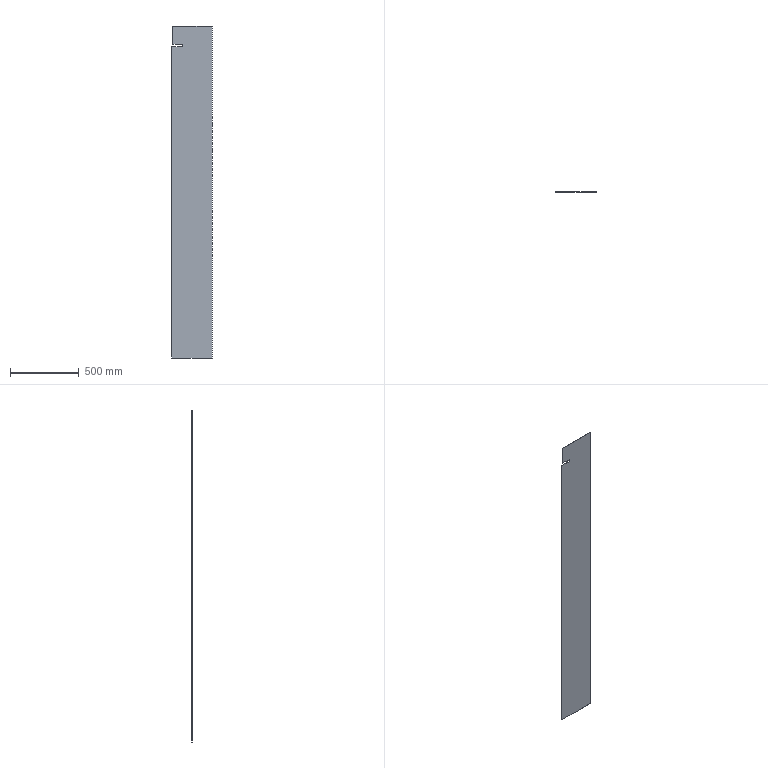Part | STEP file | E3-中转釜花纹Plate 2 | 1 solid | 11 faces | box 296 x 3 x 2420 mm | volume 2142114 mm3 | plane 10 | cylinder 1 | commonest cylinder face diameters 6 x1
STEP:
#1=CARTESIAN_POINT('',(0.,0.,0.));
#2=DIRECTION('',(0.,0.,1.));
#3=DIRECTION('',(1.,0.,0.));
#4=AXIS2_PLACEMENT_3D('',#1,#2,#3);
#5=CARTESIAN_POINT('',(0.,3.,2268.));
#6=VERTEX_POINT('',#5);
#7=CARTESIAN_POINT('',(0.,3.,0.));
#8=VERTEX_POINT('',#7);
#9=CARTESIAN_POINT('',(0.,3.,0.));
#10=DIRECTION('',(0.,0.,-1.));
#11=VECTOR('',#10,1.);
#12=LINE('',#9,#11);
#13=CARTESIAN_POINT('',(0.,3.,0.));
#14=DIRECTION('',(1.,0.,0.));
#15=DIRECTION('',(0.,0.,1.));
#16=AXIS2_PLACEMENT_3D('',#13,#14,#15);
#17=PLANE('',#16);
#18=CARTESIAN_POINT('',(0.,0.));
#19=DIRECTION('',(-1.,0.));
#20=VECTOR('',#19,1.);
#21=LINE('',#18,#20);
#22=(GEOMETRIC_REPRESENTATION_CONTEXT(2)PARAMETRIC_REPRESENTATION_CONTEXT()REPRESENTATION_CONTEXT('',''));
#23=DEFINITIONAL_REPRESENTATION('',(#21),#22);
#24=PCURVE('',#17,#23);
#25=CARTESIAN_POINT('',(0.,3.,0.));
#26=DIRECTION('',(0.,-1.,0.));
#27=DIRECTION('',(0.,0.,1.));
#28=AXIS2_PLACEMENT_3D('',#25,#26,#27);
#29=PLANE('',#28);
#30=CARTESIAN_POINT('',(0.,0.));
#31=DIRECTION('',(-1.,0.));
#32=VECTOR('',#31,1.);
#33=LINE('',#30,#32);
#34=(GEOMETRIC_REPRESENTATION_CONTEXT(2)PARAMETRIC_REPRESENTATION_CONTEXT()REPRESENTATION_CONTEXT('',''));
#35=DEFINITIONAL_REPRESENTATION('',(#33),#34);
#36=PCURVE('',#29,#35);
#37=SURFACE_CURVE('',#12,(#24,#36),.PCURVE_S1.);
#38=EDGE_CURVE('',#6,#8,#37,.T.);
#39=ORIENTED_EDGE('',*,*,#38,.T.);
#40=CARTESIAN_POINT('',(0.,0.,0.));
#41=VERTEX_POINT('',#40);
#42=CARTESIAN_POINT('',(0.,3.,0.));
#43=DIRECTION('',(0.,-1.,0.));
#44=VECTOR('',#43,1.);
#45=LINE('',#42,#44);
#46=CARTESIAN_POINT('',(0.,0.));
#47=DIRECTION('',(0.,1.));
#48=VECTOR('',#47,1.);
#49=LINE('',#46,#48);
#50=(GEOMETRIC_REPRESENTATION_CONTEXT(2)PARAMETRIC_REPRESENTATION_CONTEXT()REPRESENTATION_CONTEXT('',''));
#51=DEFINITIONAL_REPRESENTATION('',(#49),#50);
#52=PCURVE('',#17,#51);
#53=CARTESIAN_POINT('',(0.,3.,0.));
#54=DIRECTION('',(0.,0.,1.));
#55=DIRECTION('',(-1.,0.,0.));
#56=AXIS2_PLACEMENT_3D('',#53,#54,#55);
#57=PLANE('',#56);
#58=CARTESIAN_POINT('',(0.,0.));
#59=DIRECTION('',(0.,1.));
#60=VECTOR('',#59,1.);
#61=LINE('',#58,#60);
#62=(GEOMETRIC_REPRESENTATION_CONTEXT(2)PARAMETRIC_REPRESENTATION_CONTEXT()REPRESENTATION_CONTEXT('',''));
#63=DEFINITIONAL_REPRESENTATION('',(#61),#62);
#64=PCURVE('',#57,#63);
#65=SURFACE_CURVE('',#45,(#52,#64),.PCURVE_S1.);
#66=EDGE_CURVE('',#8,#41,#65,.T.);
#67=ORIENTED_EDGE('',*,*,#66,.T.);
#68=CARTESIAN_POINT('',(0.,0.,2268.));
#69=VERTEX_POINT('',#68);
#70=CARTESIAN_POINT('',(0.,0.,0.));
#71=DIRECTION('',(0.,0.,-1.));
#72=VECTOR('',#71,1.);
#73=LINE('',#70,#72);
#74=CARTESIAN_POINT('',(0.,3.));
#75=DIRECTION('',(-1.,0.));
#76=VECTOR('',#75,1.);
#77=LINE('',#74,#76);
#78=(GEOMETRIC_REPRESENTATION_CONTEXT(2)PARAMETRIC_REPRESENTATION_CONTEXT()REPRESENTATION_CONTEXT('',''));
#79=DEFINITIONAL_REPRESENTATION('',(#77),#78);
#80=PCURVE('',#17,#79);
#81=CARTESIAN_POINT('',(0.,0.,0.));
#82=DIRECTION('',(0.,-1.,0.));
#83=DIRECTION('',(0.,0.,1.));
#84=AXIS2_PLACEMENT_3D('',#81,#82,#83);
#85=PLANE('',#84);
#86=CARTESIAN_POINT('',(0.,0.));
#87=DIRECTION('',(-1.,0.));
#88=VECTOR('',#87,1.);
#89=LINE('',#86,#88);
#90=(GEOMETRIC_REPRESENTATION_CONTEXT(2)PARAMETRIC_REPRESENTATION_CONTEXT()REPRESENTATION_CONTEXT('',''));
#91=DEFINITIONAL_REPRESENTATION('',(#89),#90);
#92=PCURVE('',#85,#91);
#93=SURFACE_CURVE('',#73,(#80,#92),.PCURVE_S1.);
#94=EDGE_CURVE('',#69,#41,#93,.T.);
#95=ORIENTED_EDGE('',*,*,#94,.F.);
#96=CARTESIAN_POINT('',(0.,3.,2268.));
#97=DIRECTION('',(0.,-1.,0.));
#98=VECTOR('',#97,1.);
#99=LINE('',#96,#98);
#100=CARTESIAN_POINT('',(2268.,0.));
#101=DIRECTION('',(0.,1.));
#102=VECTOR('',#101,1.);
#103=LINE('',#100,#102);
#104=(GEOMETRIC_REPRESENTATION_CONTEXT(2)PARAMETRIC_REPRESENTATION_CONTEXT()REPRESENTATION_CONTEXT('',''));
#105=DEFINITIONAL_REPRESENTATION('',(#103),#104);
#106=PCURVE('',#17,#105);
#107=CARTESIAN_POINT('',(-82.,-600.,2268.));
#108=DIRECTION('',(0.,0.,-1.));
#109=DIRECTION('',(1.,0.,0.));
#110=AXIS2_PLACEMENT_3D('',#107,#108,#109);
#111=PLANE('',#110);
#112=CARTESIAN_POINT('',(82.,-603.));
#113=DIRECTION('',(0.,1.));
#114=VECTOR('',#113,1.);
#115=LINE('',#112,#114);
#116=(GEOMETRIC_REPRESENTATION_CONTEXT(2)PARAMETRIC_REPRESENTATION_CONTEXT()REPRESENTATION_CONTEXT('',''));
#117=DEFINITIONAL_REPRESENTATION('',(#115),#116);
#118=PCURVE('',#111,#117);
#119=SURFACE_CURVE('',#99,(#106,#118),.PCURVE_S1.);
#120=EDGE_CURVE('',#6,#69,#119,.T.);
#121=ORIENTED_EDGE('',*,*,#120,.F.);
#122=EDGE_LOOP('',(#39,#67,#95,#121));
#123=FACE_BOUND('',#122,.T.);
#124=ADVANCED_FACE('',(#123),#17,.F.);
#125=CARTESIAN_POINT('',(296.,0.,0.));
#126=VERTEX_POINT('',#125);
#127=CARTESIAN_POINT('',(0.,0.,0.));
#128=DIRECTION('',(1.,0.,0.));
#129=VECTOR('',#128,1.);
#130=LINE('',#127,#129);
#131=CARTESIAN_POINT('',(0.,3.));
#132=DIRECTION('',(-1.,0.));
#133=VECTOR('',#132,1.);
#134=LINE('',#131,#133);
#135=(GEOMETRIC_REPRESENTATION_CONTEXT(2)PARAMETRIC_REPRESENTATION_CONTEXT()REPRESENTATION_CONTEXT('',''));
#136=DEFINITIONAL_REPRESENTATION('',(#134),#135);
#137=PCURVE('',#57,#136);
#138=CARTESIAN_POINT('',(0.,0.));
#139=DIRECTION('',(0.,-1.));
#140=VECTOR('',#139,1.);
#141=LINE('',#138,#140);
#142=(GEOMETRIC_REPRESENTATION_CONTEXT(2)PARAMETRIC_REPRESENTATION_CONTEXT()REPRESENTATION_CONTEXT('',''));
#143=DEFINITIONAL_REPRESENTATION('',(#141),#142);
#144=PCURVE('',#85,#143);
#145=SURFACE_CURVE('',#130,(#137,#144),.PCURVE_S1.);
#146=EDGE_CURVE('',#41,#126,#145,.T.);
#147=ORIENTED_EDGE('',*,*,#146,.F.);
#148=ORIENTED_EDGE('',*,*,#66,.F.);
#149=CARTESIAN_POINT('',(296.,3.,0.));
#150=VERTEX_POINT('',#149);
#151=CARTESIAN_POINT('',(0.,3.,0.));
#152=DIRECTION('',(1.,0.,0.));
#153=VECTOR('',#152,1.);
#154=LINE('',#151,#153);
#155=CARTESIAN_POINT('',(0.,0.));
#156=DIRECTION('',(-1.,0.));
#157=VECTOR('',#156,1.);
#158=LINE('',#155,#157);
#159=(GEOMETRIC_REPRESENTATION_CONTEXT(2)PARAMETRIC_REPRESENTATION_CONTEXT()REPRESENTATION_CONTEXT('',''));
#160=DEFINITIONAL_REPRESENTATION('',(#158),#159);
#161=PCURVE('',#57,#160);
#162=CARTESIAN_POINT('',(0.,0.));
#163=DIRECTION('',(0.,-1.));
#164=VECTOR('',#163,1.);
#165=LINE('',#162,#164);
#166=(GEOMETRIC_REPRESENTATION_CONTEXT(2)PARAMETRIC_REPRESENTATION_CONTEXT()REPRESENTATION_CONTEXT('',''));
#167=DEFINITIONAL_REPRESENTATION('',(#165),#166);
#168=PCURVE('',#29,#167);
#169=SURFACE_CURVE('',#154,(#161,#168),.PCURVE_S1.);
#170=EDGE_CURVE('',#8,#150,#169,.T.);
#171=ORIENTED_EDGE('',*,*,#170,.T.);
#172=CARTESIAN_POINT('',(296.,3.,0.));
#173=DIRECTION('',(0.,-1.,0.));
#174=VECTOR('',#173,1.);
#175=LINE('',#172,#174);
#176=CARTESIAN_POINT('',(-296.,0.));
#177=DIRECTION('',(0.,1.));
#178=VECTOR('',#177,1.);
#179=LINE('',#176,#178);
#180=(GEOMETRIC_REPRESENTATION_CONTEXT(2)PARAMETRIC_REPRESENTATION_CONTEXT()REPRESENTATION_CONTEXT('',''));
#181=DEFINITIONAL_REPRESENTATION('',(#179),#180);
#182=PCURVE('',#57,#181);
#183=CARTESIAN_POINT('',(296.,3.,0.));
#184=DIRECTION('',(-1.,0.,0.));
#185=DIRECTION('',(0.,0.,-1.));
#186=AXIS2_PLACEMENT_3D('',#183,#184,#185);
#187=PLANE('',#186);
#188=CARTESIAN_POINT('',(0.,0.));
#189=DIRECTION('',(0.,1.));
#190=VECTOR('',#189,1.);
#191=LINE('',#188,#190);
#192=(GEOMETRIC_REPRESENTATION_CONTEXT(2)PARAMETRIC_REPRESENTATION_CONTEXT()REPRESENTATION_CONTEXT('',''));
#193=DEFINITIONAL_REPRESENTATION('',(#191),#192);
#194=PCURVE('',#187,#193);
#195=SURFACE_CURVE('',#175,(#182,#194),.PCURVE_S1.);
#196=EDGE_CURVE('',#150,#126,#195,.T.);
#197=ORIENTED_EDGE('',*,*,#196,.T.);
#198=EDGE_LOOP('',(#147,#148,#171,#197));
#199=FACE_BOUND('',#198,.T.);
#200=ADVANCED_FACE('',(#199),#57,.F.);
#201=CARTESIAN_POINT('',(296.,0.,2420.));
#202=VERTEX_POINT('',#201);
#203=CARTESIAN_POINT('',(296.,0.,0.));
#204=DIRECTION('',(0.,0.,1.));
#205=VECTOR('',#204,1.);
#206=LINE('',#203,#205);
#207=CARTESIAN_POINT('',(0.,3.));
#208=DIRECTION('',(-1.,0.));
#209=VECTOR('',#208,1.);
#210=LINE('',#207,#209);
#211=(GEOMETRIC_REPRESENTATION_CONTEXT(2)PARAMETRIC_REPRESENTATION_CONTEXT()REPRESENTATION_CONTEXT('',''));
#212=DEFINITIONAL_REPRESENTATION('',(#210),#211);
#213=PCURVE('',#187,#212);
#214=CARTESIAN_POINT('',(0.,-296.));
#215=DIRECTION('',(1.,0.));
#216=VECTOR('',#215,1.);
#217=LINE('',#214,#216);
#218=(GEOMETRIC_REPRESENTATION_CONTEXT(2)PARAMETRIC_REPRESENTATION_CONTEXT()REPRESENTATION_CONTEXT('',''));
#219=DEFINITIONAL_REPRESENTATION('',(#217),#218);
#220=PCURVE('',#85,#219);
#221=SURFACE_CURVE('',#206,(#213,#220),.PCURVE_S1.);
#222=EDGE_CURVE('',#126,#202,#221,.T.);
#223=ORIENTED_EDGE('',*,*,#222,.F.);
#224=ORIENTED_EDGE('',*,*,#196,.F.);
#225=CARTESIAN_POINT('',(296.,3.,2420.));
#226=VERTEX_POINT('',#225);
#227=CARTESIAN_POINT('',(296.,3.,0.));
#228=DIRECTION('',(0.,0.,1.));
#229=VECTOR('',#228,1.);
#230=LINE('',#227,#229);
#231=CARTESIAN_POINT('',(0.,0.));
#232=DIRECTION('',(-1.,0.));
#233=VECTOR('',#232,1.);
#234=LINE('',#231,#233);
#235=(GEOMETRIC_REPRESENTATION_CONTEXT(2)PARAMETRIC_REPRESENTATION_CONTEXT()REPRESENTATION_CONTEXT('',''));
#236=DEFINITIONAL_REPRESENTATION('',(#234),#235);
#237=PCURVE('',#187,#236);
#238=CARTESIAN_POINT('',(0.,-296.));
#239=DIRECTION('',(1.,0.));
#240=VECTOR('',#239,1.);
#241=LINE('',#238,#240);
#242=(GEOMETRIC_REPRESENTATION_CONTEXT(2)PARAMETRIC_REPRESENTATION_CONTEXT()REPRESENTATION_CONTEXT('',''));
#243=DEFINITIONAL_REPRESENTATION('',(#241),#242);
#244=PCURVE('',#29,#243);
#245=SURFACE_CURVE('',#230,(#237,#244),.PCURVE_S1.);
#246=EDGE_CURVE('',#150,#226,#245,.T.);
#247=ORIENTED_EDGE('',*,*,#246,.T.);
#248=CARTESIAN_POINT('',(296.,3.,2420.));
#249=DIRECTION('',(0.,-1.,0.));
#250=VECTOR('',#249,1.);
#251=LINE('',#248,#250);
#252=CARTESIAN_POINT('',(-2420.,0.));
#253=DIRECTION('',(0.,1.));
#254=VECTOR('',#253,1.);
#255=LINE('',#252,#254);
#256=(GEOMETRIC_REPRESENTATION_CONTEXT(2)PARAMETRIC_REPRESENTATION_CONTEXT()REPRESENTATION_CONTEXT('',''));
#257=DEFINITIONAL_REPRESENTATION('',(#255),#256);
#258=PCURVE('',#187,#257);
#259=CARTESIAN_POINT('',(0.,3.,2420.));
#260=DIRECTION('',(0.,0.,-1.));
#261=DIRECTION('',(1.,0.,0.));
#262=AXIS2_PLACEMENT_3D('',#259,#260,#261);
#263=PLANE('',#262);
#264=CARTESIAN_POINT('',(296.,0.));
#265=DIRECTION('',(0.,1.));
#266=VECTOR('',#265,1.);
#267=LINE('',#264,#266);
#268=(GEOMETRIC_REPRESENTATION_CONTEXT(2)PARAMETRIC_REPRESENTATION_CONTEXT()REPRESENTATION_CONTEXT('',''));
#269=DEFINITIONAL_REPRESENTATION('',(#267),#268);
#270=PCURVE('',#263,#269);
#271=SURFACE_CURVE('',#251,(#258,#270),.PCURVE_S1.);
#272=EDGE_CURVE('',#226,#202,#271,.T.);
#273=ORIENTED_EDGE('',*,*,#272,.T.);
#274=EDGE_LOOP('',(#223,#224,#247,#273));
#275=FACE_BOUND('',#274,.T.);
#276=ADVANCED_FACE('',(#275),#187,.F.);
#277=CARTESIAN_POINT('',(6.,0.,2420.));
#278=VERTEX_POINT('',#277);
#279=CARTESIAN_POINT('',(0.,0.,2420.));
#280=DIRECTION('',(-1.,0.,0.));
#281=VECTOR('',#280,1.);
#282=LINE('',#279,#281);
#283=CARTESIAN_POINT('',(0.,3.));
#284=DIRECTION('',(-1.,0.));
#285=VECTOR('',#284,1.);
#286=LINE('',#283,#285);
#287=(GEOMETRIC_REPRESENTATION_CONTEXT(2)PARAMETRIC_REPRESENTATION_CONTEXT()REPRESENTATION_CONTEXT('',''));
#288=DEFINITIONAL_REPRESENTATION('',(#286),#287);
#289=PCURVE('',#263,#288);
#290=CARTESIAN_POINT('',(2420.,0.));
#291=DIRECTION('',(0.,1.));
#292=VECTOR('',#291,1.);
#293=LINE('',#290,#292);
#294=(GEOMETRIC_REPRESENTATION_CONTEXT(2)PARAMETRIC_REPRESENTATION_CONTEXT()REPRESENTATION_CONTEXT('',''));
#295=DEFINITIONAL_REPRESENTATION('',(#293),#294);
#296=PCURVE('',#85,#295);
#297=SURFACE_CURVE('',#282,(#289,#296),.PCURVE_S1.);
#298=EDGE_CURVE('',#202,#278,#297,.T.);
#299=ORIENTED_EDGE('',*,*,#298,.F.);
#300=ORIENTED_EDGE('',*,*,#272,.F.);
#301=CARTESIAN_POINT('',(6.,3.,2420.));
#302=VERTEX_POINT('',#301);
#303=CARTESIAN_POINT('',(0.,3.,2420.));
#304=DIRECTION('',(-1.,0.,0.));
#305=VECTOR('',#304,1.);
#306=LINE('',#303,#305);
#307=CARTESIAN_POINT('',(0.,0.));
#308=DIRECTION('',(-1.,0.));
#309=VECTOR('',#308,1.);
#310=LINE('',#307,#309);
#311=(GEOMETRIC_REPRESENTATION_CONTEXT(2)PARAMETRIC_REPRESENTATION_CONTEXT()REPRESENTATION_CONTEXT('',''));
#312=DEFINITIONAL_REPRESENTATION('',(#310),#311);
#313=PCURVE('',#263,#312);
#314=CARTESIAN_POINT('',(2420.,0.));
#315=DIRECTION('',(0.,1.));
#316=VECTOR('',#315,1.);
#317=LINE('',#314,#316);
#318=(GEOMETRIC_REPRESENTATION_CONTEXT(2)PARAMETRIC_REPRESENTATION_CONTEXT()REPRESENTATION_CONTEXT('',''));
#319=DEFINITIONAL_REPRESENTATION('',(#317),#318);
#320=PCURVE('',#29,#319);
#321=SURFACE_CURVE('',#306,(#313,#320),.PCURVE_S1.);
#322=EDGE_CURVE('',#226,#302,#321,.T.);
#323=ORIENTED_EDGE('',*,*,#322,.T.);
#324=CARTESIAN_POINT('',(6.,3.,2420.));
#325=DIRECTION('',(0.,1.,0.));
#326=VECTOR('',#325,1.);
#327=LINE('',#324,#326);
#328=CARTESIAN_POINT('',(6.,0.));
#329=DIRECTION('',(0.,-1.));
#330=VECTOR('',#329,1.);
#331=LINE('',#328,#330);
#332=(GEOMETRIC_REPRESENTATION_CONTEXT(2)PARAMETRIC_REPRESENTATION_CONTEXT()REPRESENTATION_CONTEXT('',''));
#333=DEFINITIONAL_REPRESENTATION('',(#331),#332);
#334=PCURVE('',#263,#333);
#335=CARTESIAN_POINT('',(6.,-600.,2290.));
#336=DIRECTION('',(1.,0.,0.));
#337=DIRECTION('',(0.,0.,1.));
#338=AXIS2_PLACEMENT_3D('',#335,#336,#337);
#339=PLANE('',#338);
#340=CARTESIAN_POINT('',(130.,-603.));
#341=DIRECTION('',(0.,-1.));
#342=VECTOR('',#341,1.);
#343=LINE('',#340,#342);
#344=(GEOMETRIC_REPRESENTATION_CONTEXT(2)PARAMETRIC_REPRESENTATION_CONTEXT()REPRESENTATION_CONTEXT('',''));
#345=DEFINITIONAL_REPRESENTATION('',(#343),#344);
#346=PCURVE('',#339,#345);
#347=SURFACE_CURVE('',#327,(#334,#346),.PCURVE_S1.);
#348=EDGE_CURVE('',#278,#302,#347,.T.);
#349=ORIENTED_EDGE('',*,*,#348,.F.);
#350=EDGE_LOOP('',(#299,#300,#323,#349));
#351=FACE_BOUND('',#350,.T.);
#352=ADVANCED_FACE('',(#351),#263,.F.);
#353=ORIENTED_EDGE('',*,*,#322,.F.);
#354=ORIENTED_EDGE('',*,*,#246,.F.);
#355=ORIENTED_EDGE('',*,*,#170,.F.);
#356=ORIENTED_EDGE('',*,*,#38,.F.);
#357=CARTESIAN_POINT('',(78.,3.,2268.));
#358=VERTEX_POINT('',#357);
#359=CARTESIAN_POINT('',(0.,3.,2268.));
#360=DIRECTION('',(-1.,0.,0.));
#361=VECTOR('',#360,1.);
#362=LINE('',#359,#361);
#363=CARTESIAN_POINT('',(2268.,0.));
#364=DIRECTION('',(0.,1.));
#365=VECTOR('',#364,1.);
#366=LINE('',#363,#365);
#367=(GEOMETRIC_REPRESENTATION_CONTEXT(2)PARAMETRIC_REPRESENTATION_CONTEXT()REPRESENTATION_CONTEXT('',''));
#368=DEFINITIONAL_REPRESENTATION('',(#366),#367);
#369=PCURVE('',#29,#368);
#370=CARTESIAN_POINT('',(82.,-603.));
#371=DIRECTION('',(-1.,0.));
#372=VECTOR('',#371,1.);
#373=LINE('',#370,#372);
#374=(GEOMETRIC_REPRESENTATION_CONTEXT(2)PARAMETRIC_REPRESENTATION_CONTEXT()REPRESENTATION_CONTEXT('',''));
#375=DEFINITIONAL_REPRESENTATION('',(#373),#374);
#376=PCURVE('',#111,#375);
#377=SURFACE_CURVE('',#362,(#369,#376),.PCURVE_S1.);
#378=EDGE_CURVE('',#358,#6,#377,.T.);
#379=ORIENTED_EDGE('',*,*,#378,.F.);
#380=CARTESIAN_POINT('',(78.,3.,2287.));
#381=VERTEX_POINT('',#380);
#382=CARTESIAN_POINT('',(78.,3.,0.));
#383=DIRECTION('',(0.,0.,-1.));
#384=VECTOR('',#383,1.);
#385=LINE('',#382,#384);
#386=CARTESIAN_POINT('',(0.,-78.));
#387=DIRECTION('',(-1.,0.));
#388=VECTOR('',#387,1.);
#389=LINE('',#386,#388);
#390=(GEOMETRIC_REPRESENTATION_CONTEXT(2)PARAMETRIC_REPRESENTATION_CONTEXT()REPRESENTATION_CONTEXT('',''));
#391=DEFINITIONAL_REPRESENTATION('',(#389),#390);
#392=PCURVE('',#29,#391);
#393=CARTESIAN_POINT('',(78.,-600.,2268.));
#394=DIRECTION('',(1.,0.,0.));
#395=DIRECTION('',(0.,0.,1.));
#396=AXIS2_PLACEMENT_3D('',#393,#394,#395);
#397=PLANE('',#396);
#398=CARTESIAN_POINT('',(-2268.,-603.));
#399=DIRECTION('',(-1.,0.));
#400=VECTOR('',#399,1.);
#401=LINE('',#398,#400);
#402=(GEOMETRIC_REPRESENTATION_CONTEXT(2)PARAMETRIC_REPRESENTATION_CONTEXT()REPRESENTATION_CONTEXT('',''));
#403=DEFINITIONAL_REPRESENTATION('',(#401),#402);
#404=PCURVE('',#397,#403);
#405=SURFACE_CURVE('',#385,(#392,#404),.PCURVE_S1.);
#406=EDGE_CURVE('',#381,#358,#405,.T.);
#407=ORIENTED_EDGE('',*,*,#406,.F.);
#408=CARTESIAN_POINT('',(9.,3.,2287.));
#409=VERTEX_POINT('',#408);
#410=CARTESIAN_POINT('',(0.,3.,2287.));
#411=DIRECTION('',(1.,0.,0.));
#412=VECTOR('',#411,1.);
#413=LINE('',#410,#412);
#414=CARTESIAN_POINT('',(2287.,0.));
#415=DIRECTION('',(0.,-1.));
#416=VECTOR('',#415,1.);
#417=LINE('',#414,#416);
#418=(GEOMETRIC_REPRESENTATION_CONTEXT(2)PARAMETRIC_REPRESENTATION_CONTEXT()REPRESENTATION_CONTEXT('',''));
#419=DEFINITIONAL_REPRESENTATION('',(#417),#418);
#420=PCURVE('',#29,#419);
#421=CARTESIAN_POINT('',(78.,-600.,2287.));
#422=DIRECTION('',(0.,0.,1.));
#423=DIRECTION('',(-1.,0.,0.));
#424=AXIS2_PLACEMENT_3D('',#421,#422,#423);
#425=PLANE('',#424);
#426=CARTESIAN_POINT('',(78.,-603.));
#427=DIRECTION('',(-1.,0.));
#428=VECTOR('',#427,1.);
#429=LINE('',#426,#428);
#430=(GEOMETRIC_REPRESENTATION_CONTEXT(2)PARAMETRIC_REPRESENTATION_CONTEXT()REPRESENTATION_CONTEXT('',''));
#431=DEFINITIONAL_REPRESENTATION('',(#429),#430);
#432=PCURVE('',#425,#431);
#433=SURFACE_CURVE('',#413,(#420,#432),.PCURVE_S1.);
#434=EDGE_CURVE('',#409,#381,#433,.T.);
#435=ORIENTED_EDGE('',*,*,#434,.F.);
#436=CARTESIAN_POINT('',(6.,3.,2290.));
#437=VERTEX_POINT('',#436);
#438=CARTESIAN_POINT('',(9.,3.,2290.));
#439=DIRECTION('',(0.,-1.,0.));
#440=DIRECTION('',(0.,0.,1.));
#441=AXIS2_PLACEMENT_3D('',#438,#439,#440);
#442=CIRCLE('',#441,3.);
#443=CARTESIAN_POINT('',(2290.,-9.));
#444=DIRECTION('',(1.,0.));
#445=AXIS2_PLACEMENT_2D('',#443,#444);
#446=CIRCLE('',#445,3.);
#447=(GEOMETRIC_REPRESENTATION_CONTEXT(2)PARAMETRIC_REPRESENTATION_CONTEXT()REPRESENTATION_CONTEXT('',''));
#448=DEFINITIONAL_REPRESENTATION('',(#446),#447);
#449=PCURVE('',#29,#448);
#450=CARTESIAN_POINT('',(9.,-600.,2290.));
#451=DIRECTION('',(0.,1.,0.));
#452=DIRECTION('',(0.,0.,-1.));
#453=AXIS2_PLACEMENT_3D('',#450,#451,#452);
#454=CYLINDRICAL_SURFACE('',#453,3.);
#455=CARTESIAN_POINT('',(3.142,603.));
#456=DIRECTION('',(-1.,0.));
#457=VECTOR('',#456,1.);
#458=LINE('',#455,#457);
#459=(GEOMETRIC_REPRESENTATION_CONTEXT(2)PARAMETRIC_REPRESENTATION_CONTEXT()REPRESENTATION_CONTEXT('',''));
#460=DEFINITIONAL_REPRESENTATION('',(#458),#459);
#461=PCURVE('',#454,#460);
#462=SURFACE_CURVE('',#442,(#449,#461),.PCURVE_S1.);
#463=EDGE_CURVE('',#437,#409,#462,.T.);
#464=ORIENTED_EDGE('',*,*,#463,.F.);
#465=CARTESIAN_POINT('',(6.,3.,0.));
#466=DIRECTION('',(0.,0.,-1.));
#467=VECTOR('',#466,1.);
#468=LINE('',#465,#467);
#469=CARTESIAN_POINT('',(0.,-6.));
#470=DIRECTION('',(-1.,0.));
#471=VECTOR('',#470,1.);
#472=LINE('',#469,#471);
#473=(GEOMETRIC_REPRESENTATION_CONTEXT(2)PARAMETRIC_REPRESENTATION_CONTEXT()REPRESENTATION_CONTEXT('',''));
#474=DEFINITIONAL_REPRESENTATION('',(#472),#473);
#475=PCURVE('',#29,#474);
#476=CARTESIAN_POINT('',(-2290.,-603.));
#477=DIRECTION('',(-1.,0.));
#478=VECTOR('',#477,1.);
#479=LINE('',#476,#478);
#480=(GEOMETRIC_REPRESENTATION_CONTEXT(2)PARAMETRIC_REPRESENTATION_CONTEXT()REPRESENTATION_CONTEXT('',''));
#481=DEFINITIONAL_REPRESENTATION('',(#479),#480);
#482=PCURVE('',#339,#481);
#483=SURFACE_CURVE('',#468,(#475,#482),.PCURVE_S1.);
#484=EDGE_CURVE('',#302,#437,#483,.T.);
#485=ORIENTED_EDGE('',*,*,#484,.F.);
#486=EDGE_LOOP('',(#353,#354,#355,#356,#379,#407,#435,#464,#485));
#487=FACE_BOUND('',#486,.T.);
#488=ADVANCED_FACE('',(#487),#29,.F.);
#489=CARTESIAN_POINT('',(6.,0.,2290.));
#490=VERTEX_POINT('',#489);
#491=CARTESIAN_POINT('',(6.,0.,0.));
#492=DIRECTION('',(0.,0.,-1.));
#493=VECTOR('',#492,1.);
#494=LINE('',#491,#493);
#495=CARTESIAN_POINT('',(0.,-6.));
#496=DIRECTION('',(-1.,0.));
#497=VECTOR('',#496,1.);
#498=LINE('',#495,#497);
#499=(GEOMETRIC_REPRESENTATION_CONTEXT(2)PARAMETRIC_REPRESENTATION_CONTEXT()REPRESENTATION_CONTEXT('',''));
#500=DEFINITIONAL_REPRESENTATION('',(#498),#499);
#501=PCURVE('',#85,#500);
#502=CARTESIAN_POINT('',(-2290.,-600.));
#503=DIRECTION('',(-1.,0.));
#504=VECTOR('',#503,1.);
#505=LINE('',#502,#504);
#506=(GEOMETRIC_REPRESENTATION_CONTEXT(2)PARAMETRIC_REPRESENTATION_CONTEXT()REPRESENTATION_CONTEXT('',''));
#507=DEFINITIONAL_REPRESENTATION('',(#505),#506);
#508=PCURVE('',#339,#507);
#509=SURFACE_CURVE('',#494,(#501,#508),.PCURVE_S1.);
#510=EDGE_CURVE('',#278,#490,#509,.T.);
#511=ORIENTED_EDGE('',*,*,#510,.T.);
#512=CARTESIAN_POINT('',(9.,0.,2287.));
#513=VERTEX_POINT('',#512);
#514=CARTESIAN_POINT('',(9.,0.,2290.));
#515=DIRECTION('',(0.,-1.,0.));
#516=DIRECTION('',(0.,0.,1.));
#517=AXIS2_PLACEMENT_3D('',#514,#515,#516);
#518=CIRCLE('',#517,3.);
#519=CARTESIAN_POINT('',(2290.,-9.));
#520=DIRECTION('',(1.,0.));
#521=AXIS2_PLACEMENT_2D('',#519,#520);
#522=CIRCLE('',#521,3.);
#523=(GEOMETRIC_REPRESENTATION_CONTEXT(2)PARAMETRIC_REPRESENTATION_CONTEXT()REPRESENTATION_CONTEXT('',''));
#524=DEFINITIONAL_REPRESENTATION('',(#522),#523);
#525=PCURVE('',#85,#524);
#526=CARTESIAN_POINT('',(3.142,600.));
#527=DIRECTION('',(-1.,0.));
#528=VECTOR('',#527,1.);
#529=LINE('',#526,#528);
#530=(GEOMETRIC_REPRESENTATION_CONTEXT(2)PARAMETRIC_REPRESENTATION_CONTEXT()REPRESENTATION_CONTEXT('',''));
#531=DEFINITIONAL_REPRESENTATION('',(#529),#530);
#532=PCURVE('',#454,#531);
#533=SURFACE_CURVE('',#518,(#525,#532),.PCURVE_S1.);
#534=EDGE_CURVE('',#490,#513,#533,.T.);
#535=ORIENTED_EDGE('',*,*,#534,.T.);
#536=CARTESIAN_POINT('',(78.,0.,2287.));
#537=VERTEX_POINT('',#536);
#538=CARTESIAN_POINT('',(0.,0.,2287.));
#539=DIRECTION('',(1.,0.,0.));
#540=VECTOR('',#539,1.);
#541=LINE('',#538,#540);
#542=CARTESIAN_POINT('',(2287.,0.));
#543=DIRECTION('',(0.,-1.));
#544=VECTOR('',#543,1.);
#545=LINE('',#542,#544);
#546=(GEOMETRIC_REPRESENTATION_CONTEXT(2)PARAMETRIC_REPRESENTATION_CONTEXT()REPRESENTATION_CONTEXT('',''));
#547=DEFINITIONAL_REPRESENTATION('',(#545),#546);
#548=PCURVE('',#85,#547);
#549=CARTESIAN_POINT('',(78.,-600.));
#550=DIRECTION('',(-1.,0.));
#551=VECTOR('',#550,1.);
#552=LINE('',#549,#551);
#553=(GEOMETRIC_REPRESENTATION_CONTEXT(2)PARAMETRIC_REPRESENTATION_CONTEXT()REPRESENTATION_CONTEXT('',''));
#554=DEFINITIONAL_REPRESENTATION('',(#552),#553);
#555=PCURVE('',#425,#554);
#556=SURFACE_CURVE('',#541,(#548,#555),.PCURVE_S1.);
#557=EDGE_CURVE('',#513,#537,#556,.T.);
#558=ORIENTED_EDGE('',*,*,#557,.T.);
#559=CARTESIAN_POINT('',(78.,0.,2268.));
#560=VERTEX_POINT('',#559);
#561=CARTESIAN_POINT('',(78.,0.,0.));
#562=DIRECTION('',(0.,0.,-1.));
#563=VECTOR('',#562,1.);
#564=LINE('',#561,#563);
#565=CARTESIAN_POINT('',(0.,-78.));
#566=DIRECTION('',(-1.,0.));
#567=VECTOR('',#566,1.);
#568=LINE('',#565,#567);
#569=(GEOMETRIC_REPRESENTATION_CONTEXT(2)PARAMETRIC_REPRESENTATION_CONTEXT()REPRESENTATION_CONTEXT('',''));
#570=DEFINITIONAL_REPRESENTATION('',(#568),#569);
#571=PCURVE('',#85,#570);
#572=CARTESIAN_POINT('',(-2268.,-600.));
#573=DIRECTION('',(-1.,0.));
#574=VECTOR('',#573,1.);
#575=LINE('',#572,#574);
#576=(GEOMETRIC_REPRESENTATION_CONTEXT(2)PARAMETRIC_REPRESENTATION_CONTEXT()REPRESENTATION_CONTEXT('',''));
#577=DEFINITIONAL_REPRESENTATION('',(#575),#576);
#578=PCURVE('',#397,#577);
#579=SURFACE_CURVE('',#564,(#571,#578),.PCURVE_S1.);
#580=EDGE_CURVE('',#537,#560,#579,.T.);
#581=ORIENTED_EDGE('',*,*,#580,.T.);
#582=CARTESIAN_POINT('',(0.,0.,2268.));
#583=DIRECTION('',(-1.,0.,0.));
#584=VECTOR('',#583,1.);
#585=LINE('',#582,#584);
#586=CARTESIAN_POINT('',(2268.,0.));
#587=DIRECTION('',(0.,1.));
#588=VECTOR('',#587,1.);
#589=LINE('',#586,#588);
#590=(GEOMETRIC_REPRESENTATION_CONTEXT(2)PARAMETRIC_REPRESENTATION_CONTEXT()REPRESENTATION_CONTEXT('',''));
#591=DEFINITIONAL_REPRESENTATION('',(#589),#590);
#592=PCURVE('',#85,#591);
#593=CARTESIAN_POINT('',(82.,-600.));
#594=DIRECTION('',(-1.,0.));
#595=VECTOR('',#594,1.);
#596=LINE('',#593,#595);
#597=(GEOMETRIC_REPRESENTATION_CONTEXT(2)PARAMETRIC_REPRESENTATION_CONTEXT()REPRESENTATION_CONTEXT('',''));
#598=DEFINITIONAL_REPRESENTATION('',(#596),#597);
#599=PCURVE('',#111,#598);
#600=SURFACE_CURVE('',#585,(#592,#599),.PCURVE_S1.);
#601=EDGE_CURVE('',#560,#69,#600,.T.);
#602=ORIENTED_EDGE('',*,*,#601,.T.);
#603=ORIENTED_EDGE('',*,*,#94,.T.);
#604=ORIENTED_EDGE('',*,*,#146,.T.);
#605=ORIENTED_EDGE('',*,*,#222,.T.);
#606=ORIENTED_EDGE('',*,*,#298,.T.);
#607=EDGE_LOOP('',(#511,#535,#558,#581,#602,#603,#604,#605,#606));
#608=FACE_BOUND('',#607,.T.);
#609=ADVANCED_FACE('',(#608),#85,.T.);
#610=ORIENTED_EDGE('',*,*,#348,.T.);
#611=ORIENTED_EDGE('',*,*,#484,.T.);
#612=CARTESIAN_POINT('',(6.,-600.,2290.));
#613=DIRECTION('',(0.,1.,0.));
#614=VECTOR('',#613,1.);
#615=LINE('',#612,#614);
#616=CARTESIAN_POINT('',(0.,0.));
#617=DIRECTION('',(0.,-1.));
#618=VECTOR('',#617,1.);
#619=LINE('',#616,#618);
#620=(GEOMETRIC_REPRESENTATION_CONTEXT(2)PARAMETRIC_REPRESENTATION_CONTEXT()REPRESENTATION_CONTEXT('',''));
#621=DEFINITIONAL_REPRESENTATION('',(#619),#620);
#622=PCURVE('',#339,#621);
#623=CARTESIAN_POINT('',(1.571,0.));
#624=DIRECTION('',(0.,1.));
#625=VECTOR('',#624,1.);
#626=LINE('',#623,#625);
#627=(GEOMETRIC_REPRESENTATION_CONTEXT(2)PARAMETRIC_REPRESENTATION_CONTEXT()REPRESENTATION_CONTEXT('',''));
#628=DEFINITIONAL_REPRESENTATION('',(#626),#627);
#629=PCURVE('',#454,#628);
#630=SURFACE_CURVE('',#615,(#622,#629),.PCURVE_S1.);
#631=EDGE_CURVE('',#490,#437,#630,.T.);
#632=ORIENTED_EDGE('',*,*,#631,.F.);
#633=ORIENTED_EDGE('',*,*,#510,.F.);
#634=EDGE_LOOP('',(#610,#611,#632,#633));
#635=FACE_BOUND('',#634,.T.);
#636=ADVANCED_FACE('',(#635),#339,.F.);
#637=ORIENTED_EDGE('',*,*,#631,.T.);
#638=ORIENTED_EDGE('',*,*,#463,.T.);
#639=CARTESIAN_POINT('',(9.,-600.,2287.));
#640=DIRECTION('',(0.,1.,0.));
#641=VECTOR('',#640,1.);
#642=LINE('',#639,#641);
#643=CARTESIAN_POINT('',(0.,0.));
#644=DIRECTION('',(0.,1.));
#645=VECTOR('',#644,1.);
#646=LINE('',#643,#645);
#647=(GEOMETRIC_REPRESENTATION_CONTEXT(2)PARAMETRIC_REPRESENTATION_CONTEXT()REPRESENTATION_CONTEXT('',''));
#648=DEFINITIONAL_REPRESENTATION('',(#646),#647);
#649=PCURVE('',#454,#648);
#650=CARTESIAN_POINT('',(69.,0.));
#651=DIRECTION('',(0.,-1.));
#652=VECTOR('',#651,1.);
#653=LINE('',#650,#652);
#654=(GEOMETRIC_REPRESENTATION_CONTEXT(2)PARAMETRIC_REPRESENTATION_CONTEXT()REPRESENTATION_CONTEXT('',''));
#655=DEFINITIONAL_REPRESENTATION('',(#653),#654);
#656=PCURVE('',#425,#655);
#657=SURFACE_CURVE('',#642,(#649,#656),.PCURVE_S1.);
#658=EDGE_CURVE('',#513,#409,#657,.T.);
#659=ORIENTED_EDGE('',*,*,#658,.F.);
#660=ORIENTED_EDGE('',*,*,#534,.F.);
#661=EDGE_LOOP('',(#637,#638,#659,#660));
#662=FACE_BOUND('',#661,.T.);
#663=ADVANCED_FACE('',(#662),#454,.T.);
#664=ORIENTED_EDGE('',*,*,#658,.T.);
#665=ORIENTED_EDGE('',*,*,#434,.T.);
#666=CARTESIAN_POINT('',(78.,-600.,2287.));
#667=DIRECTION('',(0.,1.,0.));
#668=VECTOR('',#667,1.);
#669=LINE('',#666,#668);
#670=CARTESIAN_POINT('',(0.,0.));
#671=DIRECTION('',(0.,-1.));
#672=VECTOR('',#671,1.);
#673=LINE('',#670,#672);
#674=(GEOMETRIC_REPRESENTATION_CONTEXT(2)PARAMETRIC_REPRESENTATION_CONTEXT()REPRESENTATION_CONTEXT('',''));
#675=DEFINITIONAL_REPRESENTATION('',(#673),#674);
#676=PCURVE('',#425,#675);
#677=CARTESIAN_POINT('',(19.,0.));
#678=DIRECTION('',(0.,-1.));
#679=VECTOR('',#678,1.);
#680=LINE('',#677,#679);
#681=(GEOMETRIC_REPRESENTATION_CONTEXT(2)PARAMETRIC_REPRESENTATION_CONTEXT()REPRESENTATION_CONTEXT('',''));
#682=DEFINITIONAL_REPRESENTATION('',(#680),#681);
#683=PCURVE('',#397,#682);
#684=SURFACE_CURVE('',#669,(#676,#683),.PCURVE_S1.);
#685=EDGE_CURVE('',#537,#381,#684,.T.);
#686=ORIENTED_EDGE('',*,*,#685,.F.);
#687=ORIENTED_EDGE('',*,*,#557,.F.);
#688=EDGE_LOOP('',(#664,#665,#686,#687));
#689=FACE_BOUND('',#688,.T.);
#690=ADVANCED_FACE('',(#689),#425,.F.);
#691=ORIENTED_EDGE('',*,*,#685,.T.);
#692=ORIENTED_EDGE('',*,*,#406,.T.);
#693=CARTESIAN_POINT('',(78.,-600.,2268.));
#694=DIRECTION('',(0.,1.,0.));
#695=VECTOR('',#694,1.);
#696=LINE('',#693,#695);
#697=CARTESIAN_POINT('',(0.,0.));
#698=DIRECTION('',(0.,-1.));
#699=VECTOR('',#698,1.);
#700=LINE('',#697,#699);
#701=(GEOMETRIC_REPRESENTATION_CONTEXT(2)PARAMETRIC_REPRESENTATION_CONTEXT()REPRESENTATION_CONTEXT('',''));
#702=DEFINITIONAL_REPRESENTATION('',(#700),#701);
#703=PCURVE('',#397,#702);
#704=CARTESIAN_POINT('',(160.,0.));
#705=DIRECTION('',(0.,-1.));
#706=VECTOR('',#705,1.);
#707=LINE('',#704,#706);
#708=(GEOMETRIC_REPRESENTATION_CONTEXT(2)PARAMETRIC_REPRESENTATION_CONTEXT()REPRESENTATION_CONTEXT('',''));
#709=DEFINITIONAL_REPRESENTATION('',(#707),#708);
#710=PCURVE('',#111,#709);
#711=SURFACE_CURVE('',#696,(#703,#710),.PCURVE_S1.);
#712=EDGE_CURVE('',#560,#358,#711,.T.);
#713=ORIENTED_EDGE('',*,*,#712,.F.);
#714=ORIENTED_EDGE('',*,*,#580,.F.);
#715=EDGE_LOOP('',(#691,#692,#713,#714));
#716=FACE_BOUND('',#715,.T.);
#717=ADVANCED_FACE('',(#716),#397,.F.);
#718=ORIENTED_EDGE('',*,*,#712,.T.);
#719=ORIENTED_EDGE('',*,*,#378,.T.);
#720=ORIENTED_EDGE('',*,*,#120,.T.);
#721=ORIENTED_EDGE('',*,*,#601,.F.);
#722=EDGE_LOOP('',(#718,#719,#720,#721));
#723=FACE_BOUND('',#722,.T.);
#724=ADVANCED_FACE('',(#723),#111,.F.);
#725=CLOSED_SHELL('',(#124,#200,#276,#352,#488,#609,#636,#663,#690,#717,#724));
#726=MANIFOLD_SOLID_BREP('',#725);
#727=(LENGTH_UNIT()NAMED_UNIT(*)SI_UNIT(.MILLI.,.METRE.));
#728=UNCERTAINTY_MEASURE_WITH_UNIT(LENGTH_MEASURE(0.0000001),#727,'','');
#729=(NAMED_UNIT(*)PLANE_ANGLE_UNIT()SI_UNIT($,.RADIAN.));
#730=(NAMED_UNIT(*)SI_UNIT($,.STERADIAN.)SOLID_ANGLE_UNIT());
#731=(GEOMETRIC_REPRESENTATION_CONTEXT(3)GLOBAL_UNCERTAINTY_ASSIGNED_CONTEXT((#728))GLOBAL_UNIT_ASSIGNED_CONTEXT((#727,#729,#730))REPRESENTATION_CONTEXT('',''));
#732=ADVANCED_BREP_SHAPE_REPRESENTATION('',(#4,#726),#731);